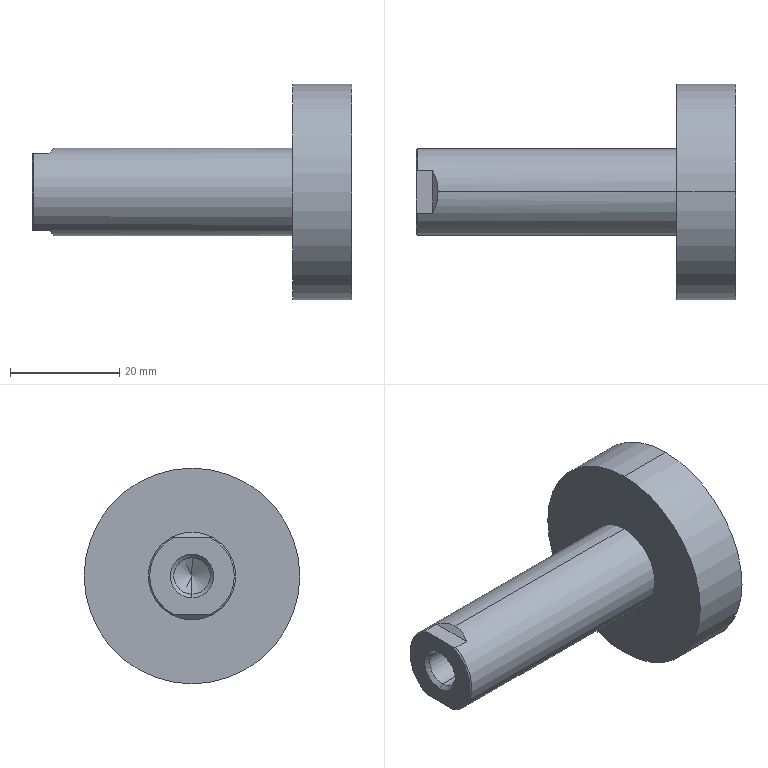Part | SolidWorks | features MBimport 1 | 1 solid | 19 faces | box 58.5 x 39.5 x 39.5 mm | volume 22261 mm3 | plane 7 | cylinder 6 | cone 6 | commonest cylinder face diameters 6.647 x2 16 x2 39.5 x2
STEP:
#1=CARTESIAN_POINT('',(-3.,0.,8.));
#2=VERTEX_POINT('',#1);
#3=CARTESIAN_POINT('',(-4.,3.873,7.));
#4=VERTEX_POINT('',#3);
#5=CARTESIAN_POINT('',(-3.,0.,8.));
#6=CARTESIAN_POINT('',(-3.,1.362,8.));
#7=CARTESIAN_POINT('',(-3.341,2.681,7.659));
#8=CARTESIAN_POINT('',(-4.,3.873,7.));
#9=(BOUNDED_CURVE()B_SPLINE_CURVE(3,(#5,#6,#7,#8),.UNSPECIFIED.,.F.,.F.)B_SPLINE_CURVE_WITH_KNOTS((4,4),(0.,0.5054),.UNSPECIFIED.)CURVE()GEOMETRIC_REPRESENTATION_ITEM()RATIONAL_B_SPLINE_CURVE((1.,0.9788,0.9788,1.))REPRESENTATION_ITEM(''));
#10=EDGE_CURVE('',#2,#4,#9,.T.);
#11=ORIENTED_EDGE('',*,*,#10,.F.);
#12=CARTESIAN_POINT('',(40.7,0.,8.));
#13=VERTEX_POINT('',#12);
#14=CARTESIAN_POINT('',(0.,0.,8.));
#15=DIRECTION('',(1.,0.,0.));
#16=VECTOR('',#15,1000.);
#17=LINE('',#14,#16);
#18=EDGE_CURVE('',#2,#13,#17,.T.);
#19=ORIENTED_EDGE('',*,*,#18,.T.);
#20=CARTESIAN_POINT('',(40.7,0.,-8.));
#21=VERTEX_POINT('',#20);
#22=CARTESIAN_POINT('',(40.7,0.,0.));
#23=DIRECTION('',(1.,0.,0.));
#24=DIRECTION('',(0.,0.,-1.));
#25=AXIS2_PLACEMENT_3D('',#22,#23,#24);
#26=CIRCLE('',#25,8.);
#27=EDGE_CURVE('',#21,#13,#26,.T.);
#28=ORIENTED_EDGE('',*,*,#27,.F.);
#29=CARTESIAN_POINT('',(-3.,0.,-8.));
#30=VERTEX_POINT('',#29);
#31=CARTESIAN_POINT('',(0.,0.,-8.));
#32=DIRECTION('',(1.,0.,0.));
#33=VECTOR('',#32,1000.);
#34=LINE('',#31,#33);
#35=EDGE_CURVE('',#30,#21,#34,.T.);
#36=ORIENTED_EDGE('',*,*,#35,.F.);
#37=CARTESIAN_POINT('',(-4.,3.873,-7.));
#38=VERTEX_POINT('',#37);
#39=CARTESIAN_POINT('',(-4.,3.873,-7.));
#40=CARTESIAN_POINT('',(-3.341,2.681,-7.659));
#41=CARTESIAN_POINT('',(-3.,1.362,-8.));
#42=CARTESIAN_POINT('',(-3.,0.,-8.));
#43=(BOUNDED_CURVE()B_SPLINE_CURVE(3,(#39,#40,#41,#42),.UNSPECIFIED.,.F.,.F.)B_SPLINE_CURVE_WITH_KNOTS((4,4),(5.778,6.283),.UNSPECIFIED.)CURVE()GEOMETRIC_REPRESENTATION_ITEM()RATIONAL_B_SPLINE_CURVE((1.,0.9788,0.9788,1.))REPRESENTATION_ITEM(''));
#44=EDGE_CURVE('',#38,#30,#43,.T.);
#45=ORIENTED_EDGE('',*,*,#44,.F.);
#46=CARTESIAN_POINT('',(-6.75,3.873,-7.));
#47=VERTEX_POINT('',#46);
#48=CARTESIAN_POINT('',(0.,3.873,-7.));
#49=DIRECTION('',(1.,0.,0.));
#50=VECTOR('',#49,1000.);
#51=LINE('',#48,#50);
#52=EDGE_CURVE('',#47,#38,#51,.T.);
#53=ORIENTED_EDGE('',*,*,#52,.F.);
#54=CARTESIAN_POINT('',(-6.75,3.873,7.));
#55=VERTEX_POINT('',#54);
#56=CARTESIAN_POINT('',(-6.75,0.,0.));
#57=DIRECTION('',(1.,0.,0.));
#58=DIRECTION('',(0.,0.,-1.));
#59=AXIS2_PLACEMENT_3D('',#56,#57,#58);
#60=CIRCLE('',#59,8.);
#61=EDGE_CURVE('',#47,#55,#60,.T.);
#62=ORIENTED_EDGE('',*,*,#61,.T.);
#63=CARTESIAN_POINT('',(0.,3.873,7.));
#64=DIRECTION('',(-1.,0.,0.));
#65=VECTOR('',#64,1000.);
#66=LINE('',#63,#65);
#67=EDGE_CURVE('',#4,#55,#66,.T.);
#68=ORIENTED_EDGE('',*,*,#67,.F.);
#69=EDGE_LOOP('',(#11,#19,#28,#36,#45,#53,#62,#68));
#70=FACE_OUTER_BOUND('',#69,.T.);
#71=CARTESIAN_POINT('',(0.,0.,0.));
#72=DIRECTION('',(1.,0.,0.));
#73=DIRECTION('',(0.,0.,-1.));
#74=AXIS2_PLACEMENT_3D('',#71,#72,#73);
#75=CYLINDRICAL_SURFACE('',#74,8.);
#76=ADVANCED_FACE('',(#70),#75,.T.);
#77=CARTESIAN_POINT('',(40.7,0.,-19.75));
#78=VERTEX_POINT('',#77);
#79=CARTESIAN_POINT('',(40.7,0.,19.75));
#80=VERTEX_POINT('',#79);
#81=CARTESIAN_POINT('',(40.7,0.,0.));
#82=DIRECTION('',(1.,0.,0.));
#83=DIRECTION('',(0.,0.,-1.));
#84=AXIS2_PLACEMENT_3D('',#81,#82,#83);
#85=CIRCLE('',#84,19.75);
#86=EDGE_CURVE('',#78,#80,#85,.T.);
#87=ORIENTED_EDGE('',*,*,#86,.T.);
#88=CARTESIAN_POINT('',(51.5,0.,19.75));
#89=VERTEX_POINT('',#88);
#90=CARTESIAN_POINT('',(51.5,0.,19.75));
#91=DIRECTION('',(1.,0.,0.));
#92=VECTOR('',#91,1000.);
#93=LINE('',#90,#92);
#94=EDGE_CURVE('',#80,#89,#93,.T.);
#95=ORIENTED_EDGE('',*,*,#94,.T.);
#96=CARTESIAN_POINT('',(51.5,0.,-19.75));
#97=VERTEX_POINT('',#96);
#98=CARTESIAN_POINT('',(51.5,0.,0.));
#99=DIRECTION('',(1.,0.,0.));
#100=DIRECTION('',(0.,0.,-1.));
#101=AXIS2_PLACEMENT_3D('',#98,#99,#100);
#102=CIRCLE('',#101,19.75);
#103=EDGE_CURVE('',#97,#89,#102,.T.);
#104=ORIENTED_EDGE('',*,*,#103,.F.);
#105=CARTESIAN_POINT('',(51.5,0.,-19.75));
#106=DIRECTION('',(1.,0.,0.));
#107=VECTOR('',#106,1000.);
#108=LINE('',#105,#107);
#109=EDGE_CURVE('',#78,#97,#108,.T.);
#110=ORIENTED_EDGE('',*,*,#109,.F.);
#111=EDGE_LOOP('',(#87,#95,#104,#110));
#112=FACE_OUTER_BOUND('',#111,.T.);
#113=CARTESIAN_POINT('',(51.5,0.,0.));
#114=DIRECTION('',(1.,0.,0.));
#115=DIRECTION('',(0.,0.,-1.));
#116=AXIS2_PLACEMENT_3D('',#113,#114,#115);
#117=CYLINDRICAL_SURFACE('',#116,19.75);
#118=ADVANCED_FACE('',(#112),#117,.T.);
#119=CARTESIAN_POINT('',(-6.324,0.,3.324));
#120=VERTEX_POINT('',#119);
#121=CARTESIAN_POINT('',(-6.324,0.,-3.324));
#122=VERTEX_POINT('',#121);
#123=CARTESIAN_POINT('',(-6.324,0.,0.));
#124=DIRECTION('',(1.,0.,0.));
#125=DIRECTION('',(0.,0.,-1.));
#126=AXIS2_PLACEMENT_3D('',#123,#124,#125);
#127=CIRCLE('',#126,3.324);
#128=EDGE_CURVE('',#120,#122,#127,.T.);
#129=ORIENTED_EDGE('',*,*,#128,.T.);
#130=CARTESIAN_POINT('',(-7.,0.,-4.));
#131=VERTEX_POINT('',#130);
#132=CARTESIAN_POINT('',(-7.,0.,-4.));
#133=DIRECTION('',(-0.7071,0.,-0.7071));
#134=VECTOR('',#133,1000.);
#135=LINE('',#132,#134);
#136=EDGE_CURVE('',#122,#131,#135,.T.);
#137=ORIENTED_EDGE('',*,*,#136,.T.);
#138=CARTESIAN_POINT('',(-7.,0.,4.));
#139=VERTEX_POINT('',#138);
#140=CARTESIAN_POINT('',(-7.,0.,0.));
#141=DIRECTION('',(1.,0.,0.));
#142=DIRECTION('',(0.,0.,-1.));
#143=AXIS2_PLACEMENT_3D('',#140,#141,#142);
#144=CIRCLE('',#143,4.);
#145=EDGE_CURVE('',#139,#131,#144,.T.);
#146=ORIENTED_EDGE('',*,*,#145,.F.);
#147=CARTESIAN_POINT('',(-7.,0.,4.));
#148=DIRECTION('',(-0.7071,0.,0.7071));
#149=VECTOR('',#148,1000.);
#150=LINE('',#147,#149);
#151=EDGE_CURVE('',#120,#139,#150,.T.);
#152=ORIENTED_EDGE('',*,*,#151,.F.);
#153=EDGE_LOOP('',(#129,#137,#146,#152));
#154=FACE_OUTER_BOUND('',#153,.T.);
#155=CARTESIAN_POINT('',(-7.,0.,0.));
#156=DIRECTION('',(-1.,0.,0.));
#157=DIRECTION('',(0.,0.,1.));
#158=AXIS2_PLACEMENT_3D('',#155,#156,#157);
#159=CONICAL_SURFACE('',#158,4.,0.7854);
#160=ADVANCED_FACE('',(#154),#159,.F.);
#161=ORIENTED_EDGE('',*,*,#128,.F.);
#162=CARTESIAN_POINT('',(7.4,0.,3.324));
#163=VERTEX_POINT('',#162);
#164=CARTESIAN_POINT('',(9.319,0.,3.324));
#165=DIRECTION('',(1.,0.,0.));
#166=VECTOR('',#165,1000.);
#167=LINE('',#164,#166);
#168=EDGE_CURVE('',#120,#163,#167,.T.);
#169=ORIENTED_EDGE('',*,*,#168,.T.);
#170=CARTESIAN_POINT('',(7.4,0.,-3.324));
#171=VERTEX_POINT('',#170);
#172=CARTESIAN_POINT('',(7.4,0.,0.));
#173=DIRECTION('',(1.,0.,0.));
#174=DIRECTION('',(0.,0.,-1.));
#175=AXIS2_PLACEMENT_3D('',#172,#173,#174);
#176=CIRCLE('',#175,3.324);
#177=EDGE_CURVE('',#163,#171,#176,.T.);
#178=ORIENTED_EDGE('',*,*,#177,.T.);
#179=CARTESIAN_POINT('',(9.319,0.,-3.324));
#180=DIRECTION('',(1.,0.,0.));
#181=VECTOR('',#180,1000.);
#182=LINE('',#179,#181);
#183=EDGE_CURVE('',#122,#171,#182,.T.);
#184=ORIENTED_EDGE('',*,*,#183,.F.);
#185=EDGE_LOOP('',(#161,#169,#178,#184));
#186=FACE_OUTER_BOUND('',#185,.T.);
#187=CARTESIAN_POINT('',(9.319,0.,0.));
#188=DIRECTION('',(1.,0.,0.));
#189=DIRECTION('',(0.,0.,-1.));
#190=AXIS2_PLACEMENT_3D('',#187,#188,#189);
#191=CYLINDRICAL_SURFACE('',#190,3.324);
#192=ADVANCED_FACE('',(#186),#191,.F.);
#193=CARTESIAN_POINT('',(9.319,0.,0.));
#194=VERTEX_POINT('',#193);
#195=CARTESIAN_POINT('',(7.4,0.,3.324));
#196=DIRECTION('',(-0.5,0.,0.866));
#197=VECTOR('',#196,1000.);
#198=LINE('',#195,#197);
#199=EDGE_CURVE('',#194,#163,#198,.T.);
#200=ORIENTED_EDGE('',*,*,#199,.F.);
#201=CARTESIAN_POINT('',(7.4,0.,-3.324));
#202=DIRECTION('',(-0.5,0.,-0.866));
#203=VECTOR('',#202,1000.);
#204=LINE('',#201,#203);
#205=EDGE_CURVE('',#194,#171,#204,.T.);
#206=ORIENTED_EDGE('',*,*,#205,.T.);
#207=ORIENTED_EDGE('',*,*,#177,.F.);
#208=EDGE_LOOP('',(#200,#206,#207));
#209=FACE_OUTER_BOUND('',#208,.T.);
#210=CARTESIAN_POINT('',(7.4,0.,0.));
#211=DIRECTION('',(-1.,0.,0.));
#212=DIRECTION('',(0.,0.,1.));
#213=AXIS2_PLACEMENT_3D('',#210,#211,#212);
#214=CONICAL_SURFACE('',#213,3.324,1.047);
#215=ADVANCED_FACE('',(#209),#214,.F.);
#216=ORIENTED_EDGE('',*,*,#205,.F.);
#217=ORIENTED_EDGE('',*,*,#199,.T.);
#218=CARTESIAN_POINT('',(7.4,0.,0.));
#219=DIRECTION('',(1.,0.,0.));
#220=DIRECTION('',(0.,0.,-1.));
#221=AXIS2_PLACEMENT_3D('',#218,#219,#220);
#222=CIRCLE('',#221,3.324);
#223=EDGE_CURVE('',#171,#163,#222,.T.);
#224=ORIENTED_EDGE('',*,*,#223,.F.);
#225=EDGE_LOOP('',(#216,#217,#224));
#226=FACE_OUTER_BOUND('',#225,.T.);
#227=CARTESIAN_POINT('',(7.4,0.,0.));
#228=DIRECTION('',(-1.,0.,0.));
#229=DIRECTION('',(0.,0.,1.));
#230=AXIS2_PLACEMENT_3D('',#227,#228,#229);
#231=CONICAL_SURFACE('',#230,3.324,1.047);
#232=ADVANCED_FACE('',(#226),#231,.F.);
#233=ORIENTED_EDGE('',*,*,#168,.F.);
#234=CARTESIAN_POINT('',(-6.324,0.,0.));
#235=DIRECTION('',(1.,0.,0.));
#236=DIRECTION('',(0.,0.,-1.));
#237=AXIS2_PLACEMENT_3D('',#234,#235,#236);
#238=CIRCLE('',#237,3.324);
#239=EDGE_CURVE('',#122,#120,#238,.T.);
#240=ORIENTED_EDGE('',*,*,#239,.F.);
#241=ORIENTED_EDGE('',*,*,#183,.T.);
#242=ORIENTED_EDGE('',*,*,#223,.T.);
#243=EDGE_LOOP('',(#233,#240,#241,#242));
#244=FACE_OUTER_BOUND('',#243,.T.);
#245=CARTESIAN_POINT('',(9.319,0.,0.));
#246=DIRECTION('',(1.,0.,0.));
#247=DIRECTION('',(0.,0.,-1.));
#248=AXIS2_PLACEMENT_3D('',#245,#246,#247);
#249=CYLINDRICAL_SURFACE('',#248,3.324);
#250=ADVANCED_FACE('',(#244),#249,.F.);
#251=ORIENTED_EDGE('',*,*,#136,.F.);
#252=ORIENTED_EDGE('',*,*,#239,.T.);
#253=ORIENTED_EDGE('',*,*,#151,.T.);
#254=CARTESIAN_POINT('',(-7.,0.,0.));
#255=DIRECTION('',(1.,0.,0.));
#256=DIRECTION('',(0.,0.,-1.));
#257=AXIS2_PLACEMENT_3D('',#254,#255,#256);
#258=CIRCLE('',#257,4.);
#259=EDGE_CURVE('',#131,#139,#258,.T.);
#260=ORIENTED_EDGE('',*,*,#259,.F.);
#261=EDGE_LOOP('',(#251,#252,#253,#260));
#262=FACE_OUTER_BOUND('',#261,.T.);
#263=CARTESIAN_POINT('',(-7.,0.,0.));
#264=DIRECTION('',(-1.,0.,0.));
#265=DIRECTION('',(0.,0.,1.));
#266=AXIS2_PLACEMENT_3D('',#263,#264,#265);
#267=CONICAL_SURFACE('',#266,4.,0.7854);
#268=ADVANCED_FACE('',(#262),#267,.F.);
#269=CARTESIAN_POINT('',(-7.,-3.326,7.));
#270=VERTEX_POINT('',#269);
#271=CARTESIAN_POINT('',(-6.75,-3.873,7.));
#272=VERTEX_POINT('',#271);
#273=CARTESIAN_POINT('',(-7.,-3.326,7.));
#274=CARTESIAN_POINT('',(-6.921,-3.51,7.));
#275=CARTESIAN_POINT('',(-6.837,-3.692,7.));
#276=CARTESIAN_POINT('',(-6.75,-3.873,7.));
#277=B_SPLINE_CURVE_WITH_KNOTS('',3,(#273,#274,#275,#276),.UNSPECIFIED.,.F.,.F.,(4,4),(0.007395,0.007986),.UNSPECIFIED.);
#278=EDGE_CURVE('',#270,#272,#277,.T.);
#279=ORIENTED_EDGE('',*,*,#278,.T.);
#280=CARTESIAN_POINT('',(-4.,-3.873,7.));
#281=VERTEX_POINT('',#280);
#282=CARTESIAN_POINT('',(0.,-3.873,7.));
#283=DIRECTION('',(1.,0.,0.));
#284=VECTOR('',#283,1000.);
#285=LINE('',#282,#284);
#286=EDGE_CURVE('',#272,#281,#285,.T.);
#287=ORIENTED_EDGE('',*,*,#286,.T.);
#288=CARTESIAN_POINT('',(-4.,14.,7.));
#289=DIRECTION('',(0.,-1.,0.));
#290=VECTOR('',#289,1000.);
#291=LINE('',#288,#290);
#292=EDGE_CURVE('',#4,#281,#291,.T.);
#293=ORIENTED_EDGE('',*,*,#292,.F.);
#294=ORIENTED_EDGE('',*,*,#67,.T.);
#295=CARTESIAN_POINT('',(-7.,3.326,7.));
#296=VERTEX_POINT('',#295);
#297=CARTESIAN_POINT('',(-6.75,3.873,7.));
#298=CARTESIAN_POINT('',(-6.838,3.692,7.));
#299=CARTESIAN_POINT('',(-6.921,3.51,7.));
#300=CARTESIAN_POINT('',(-7.,3.326,7.));
#301=B_SPLINE_CURVE_WITH_KNOTS('',3,(#297,#298,#299,#300),.UNSPECIFIED.,.F.,.F.,(4,4),(0.000001583,0.0005965),.UNSPECIFIED.);
#302=EDGE_CURVE('',#55,#296,#301,.T.);
#303=ORIENTED_EDGE('',*,*,#302,.T.);
#304=CARTESIAN_POINT('',(-7.,14.,7.));
#305=DIRECTION('',(0.,-1.,0.));
#306=VECTOR('',#305,1000.);
#307=LINE('',#304,#306);
#308=EDGE_CURVE('',#296,#270,#307,.T.);
#309=ORIENTED_EDGE('',*,*,#308,.T.);
#310=EDGE_LOOP('',(#279,#287,#293,#294,#303,#309));
#311=FACE_OUTER_BOUND('',#310,.T.);
#312=CARTESIAN_POINT('',(-4.,14.,7.));
#313=DIRECTION('',(0.,0.,1.));
#314=DIRECTION('',(1.,0.,0.));
#315=AXIS2_PLACEMENT_3D('',#312,#313,#314);
#316=PLANE('',#315);
#317=ADVANCED_FACE('',(#311),#316,.T.);
#318=CARTESIAN_POINT('',(-4.,-3.873,7.));
#319=CARTESIAN_POINT('',(-3.341,-2.681,7.659));
#320=CARTESIAN_POINT('',(-3.,-1.362,8.));
#321=CARTESIAN_POINT('',(-3.,0.,8.));
#322=(BOUNDED_CURVE()B_SPLINE_CURVE(3,(#318,#319,#320,#321),.UNSPECIFIED.,.F.,.F.)B_SPLINE_CURVE_WITH_KNOTS((4,4),(5.778,6.283),.UNSPECIFIED.)CURVE()GEOMETRIC_REPRESENTATION_ITEM()RATIONAL_B_SPLINE_CURVE((1.,0.9788,0.9788,1.))REPRESENTATION_ITEM(''));
#323=EDGE_CURVE('',#281,#2,#322,.T.);
#324=ORIENTED_EDGE('',*,*,#323,.T.);
#325=ORIENTED_EDGE('',*,*,#10,.T.);
#326=ORIENTED_EDGE('',*,*,#292,.T.);
#327=EDGE_LOOP('',(#324,#325,#326));
#328=FACE_OUTER_BOUND('',#327,.T.);
#329=CARTESIAN_POINT('',(1.,14.,12.));
#330=DIRECTION('',(-0.7071,0.,0.7071));
#331=DIRECTION('',(0.,1.,0.));
#332=AXIS2_PLACEMENT_3D('',#329,#330,#331);
#333=PLANE('',#332);
#334=ADVANCED_FACE('',(#328),#333,.T.);
#335=CARTESIAN_POINT('',(-7.,3.326,-7.));
#336=VERTEX_POINT('',#335);
#337=CARTESIAN_POINT('',(-7.,3.326,-7.));
#338=CARTESIAN_POINT('',(-6.921,3.51,-7.));
#339=CARTESIAN_POINT('',(-6.837,3.692,-7.));
#340=CARTESIAN_POINT('',(-6.75,3.873,-7.));
#341=B_SPLINE_CURVE_WITH_KNOTS('',3,(#337,#338,#339,#340),.UNSPECIFIED.,.F.,.F.,(4,4),(0.007395,0.007986),.UNSPECIFIED.);
#342=EDGE_CURVE('',#336,#47,#341,.T.);
#343=ORIENTED_EDGE('',*,*,#342,.T.);
#344=ORIENTED_EDGE('',*,*,#52,.T.);
#345=CARTESIAN_POINT('',(-4.,-3.873,-7.));
#346=VERTEX_POINT('',#345);
#347=CARTESIAN_POINT('',(-4.,14.,-7.));
#348=DIRECTION('',(0.,-1.,0.));
#349=VECTOR('',#348,1000.);
#350=LINE('',#347,#349);
#351=EDGE_CURVE('',#38,#346,#350,.T.);
#352=ORIENTED_EDGE('',*,*,#351,.T.);
#353=CARTESIAN_POINT('',(-6.75,-3.873,-7.));
#354=VERTEX_POINT('',#353);
#355=CARTESIAN_POINT('',(0.,-3.873,-7.));
#356=DIRECTION('',(-1.,0.,0.));
#357=VECTOR('',#356,1000.);
#358=LINE('',#355,#357);
#359=EDGE_CURVE('',#346,#354,#358,.T.);
#360=ORIENTED_EDGE('',*,*,#359,.T.);
#361=CARTESIAN_POINT('',(-7.,-3.326,-7.));
#362=VERTEX_POINT('',#361);
#363=CARTESIAN_POINT('',(-6.75,-3.873,-7.));
#364=CARTESIAN_POINT('',(-6.838,-3.692,-7.));
#365=CARTESIAN_POINT('',(-6.921,-3.51,-7.));
#366=CARTESIAN_POINT('',(-7.,-3.326,-7.));
#367=B_SPLINE_CURVE_WITH_KNOTS('',3,(#363,#364,#365,#366),.UNSPECIFIED.,.F.,.F.,(4,4),(0.000001583,0.0005965),.UNSPECIFIED.);
#368=EDGE_CURVE('',#354,#362,#367,.T.);
#369=ORIENTED_EDGE('',*,*,#368,.T.);
#370=CARTESIAN_POINT('',(-7.,14.,-7.));
#371=DIRECTION('',(0.,-1.,0.));
#372=VECTOR('',#371,1000.);
#373=LINE('',#370,#372);
#374=EDGE_CURVE('',#336,#362,#373,.T.);
#375=ORIENTED_EDGE('',*,*,#374,.F.);
#376=EDGE_LOOP('',(#343,#344,#352,#360,#369,#375));
#377=FACE_OUTER_BOUND('',#376,.T.);
#378=CARTESIAN_POINT('',(-7.,14.,-7.));
#379=DIRECTION('',(0.,0.,-1.));
#380=DIRECTION('',(0.,-1.,0.));
#381=AXIS2_PLACEMENT_3D('',#378,#379,#380);
#382=PLANE('',#381);
#383=ADVANCED_FACE('',(#377),#382,.T.);
#384=ORIENTED_EDGE('',*,*,#44,.T.);
#385=CARTESIAN_POINT('',(-3.,0.,-8.));
#386=CARTESIAN_POINT('',(-3.,-1.362,-8.));
#387=CARTESIAN_POINT('',(-3.341,-2.681,-7.659));
#388=CARTESIAN_POINT('',(-4.,-3.873,-7.));
#389=(BOUNDED_CURVE()B_SPLINE_CURVE(3,(#385,#386,#387,#388),.UNSPECIFIED.,.F.,.F.)B_SPLINE_CURVE_WITH_KNOTS((4,4),(0.,0.5054),.UNSPECIFIED.)CURVE()GEOMETRIC_REPRESENTATION_ITEM()RATIONAL_B_SPLINE_CURVE((1.,0.9788,0.9788,1.))REPRESENTATION_ITEM(''));
#390=EDGE_CURVE('',#30,#346,#389,.T.);
#391=ORIENTED_EDGE('',*,*,#390,.T.);
#392=ORIENTED_EDGE('',*,*,#351,.F.);
#393=EDGE_LOOP('',(#384,#391,#392));
#394=FACE_OUTER_BOUND('',#393,.T.);
#395=CARTESIAN_POINT('',(-4.,14.,-7.));
#396=DIRECTION('',(-0.7071,0.,-0.7071));
#397=DIRECTION('',(-0.7071,0.,0.7071));
#398=AXIS2_PLACEMENT_3D('',#395,#396,#397);
#399=PLANE('',#398);
#400=ADVANCED_FACE('',(#394),#399,.T.);
#401=ORIENTED_EDGE('',*,*,#103,.T.);
#402=CARTESIAN_POINT('',(51.5,0.,0.));
#403=DIRECTION('',(1.,0.,0.));
#404=DIRECTION('',(0.,0.,-1.));
#405=AXIS2_PLACEMENT_3D('',#402,#403,#404);
#406=CIRCLE('',#405,19.75);
#407=EDGE_CURVE('',#89,#97,#406,.T.);
#408=ORIENTED_EDGE('',*,*,#407,.T.);
#409=EDGE_LOOP('',(#401,#408));
#410=FACE_OUTER_BOUND('',#409,.T.);
#411=CARTESIAN_POINT('',(51.5,19.75,0.));
#412=DIRECTION('',(-1.,0.,0.));
#413=DIRECTION('',(0.,0.,1.));
#414=AXIS2_PLACEMENT_3D('',#411,#412,#413);
#415=PLANE('',#414);
#416=ADVANCED_FACE('',(#410),#415,.F.);
#417=ORIENTED_EDGE('',*,*,#94,.F.);
#418=CARTESIAN_POINT('',(40.7,0.,0.));
#419=DIRECTION('',(1.,0.,0.));
#420=DIRECTION('',(0.,0.,-1.));
#421=AXIS2_PLACEMENT_3D('',#418,#419,#420);
#422=CIRCLE('',#421,19.75);
#423=EDGE_CURVE('',#80,#78,#422,.T.);
#424=ORIENTED_EDGE('',*,*,#423,.T.);
#425=ORIENTED_EDGE('',*,*,#109,.T.);
#426=ORIENTED_EDGE('',*,*,#407,.F.);
#427=EDGE_LOOP('',(#417,#424,#425,#426));
#428=FACE_OUTER_BOUND('',#427,.T.);
#429=CARTESIAN_POINT('',(51.5,0.,0.));
#430=DIRECTION('',(1.,0.,0.));
#431=DIRECTION('',(0.,0.,-1.));
#432=AXIS2_PLACEMENT_3D('',#429,#430,#431);
#433=CYLINDRICAL_SURFACE('',#432,19.75);
#434=ADVANCED_FACE('',(#428),#433,.T.);
#435=ORIENTED_EDGE('',*,*,#27,.T.);
#436=CARTESIAN_POINT('',(40.7,0.,0.));
#437=DIRECTION('',(1.,0.,0.));
#438=DIRECTION('',(0.,0.,-1.));
#439=AXIS2_PLACEMENT_3D('',#436,#437,#438);
#440=CIRCLE('',#439,8.);
#441=EDGE_CURVE('',#13,#21,#440,.T.);
#442=ORIENTED_EDGE('',*,*,#441,.T.);
#443=EDGE_LOOP('',(#435,#442));
#444=FACE_BOUND('',#443,.T.);
#445=ORIENTED_EDGE('',*,*,#86,.F.);
#446=ORIENTED_EDGE('',*,*,#423,.F.);
#447=EDGE_LOOP('',(#445,#446));
#448=FACE_OUTER_BOUND('',#447,.T.);
#449=CARTESIAN_POINT('',(40.7,8.,0.));
#450=DIRECTION('',(1.,0.,0.));
#451=DIRECTION('',(0.,1.,0.));
#452=AXIS2_PLACEMENT_3D('',#449,#450,#451);
#453=PLANE('',#452);
#454=ADVANCED_FACE('',(#444,#448),#453,.F.);
#455=ORIENTED_EDGE('',*,*,#18,.F.);
#456=ORIENTED_EDGE('',*,*,#323,.F.);
#457=ORIENTED_EDGE('',*,*,#286,.F.);
#458=CARTESIAN_POINT('',(-6.75,0.,0.));
#459=DIRECTION('',(1.,0.,0.));
#460=DIRECTION('',(0.,0.,-1.));
#461=AXIS2_PLACEMENT_3D('',#458,#459,#460);
#462=CIRCLE('',#461,8.);
#463=EDGE_CURVE('',#272,#354,#462,.T.);
#464=ORIENTED_EDGE('',*,*,#463,.T.);
#465=ORIENTED_EDGE('',*,*,#359,.F.);
#466=ORIENTED_EDGE('',*,*,#390,.F.);
#467=ORIENTED_EDGE('',*,*,#35,.T.);
#468=ORIENTED_EDGE('',*,*,#441,.F.);
#469=EDGE_LOOP('',(#455,#456,#457,#464,#465,#466,#467,#468));
#470=FACE_OUTER_BOUND('',#469,.T.);
#471=CARTESIAN_POINT('',(0.,0.,0.));
#472=DIRECTION('',(1.,0.,0.));
#473=DIRECTION('',(0.,0.,-1.));
#474=AXIS2_PLACEMENT_3D('',#471,#472,#473);
#475=CYLINDRICAL_SURFACE('',#474,8.);
#476=ADVANCED_FACE('',(#470),#475,.T.);
#477=ORIENTED_EDGE('',*,*,#342,.F.);
#478=CARTESIAN_POINT('',(-7.,0.,0.));
#479=DIRECTION('',(1.,0.,0.));
#480=DIRECTION('',(0.,0.,-1.));
#481=AXIS2_PLACEMENT_3D('',#478,#479,#480);
#482=CIRCLE('',#481,7.75);
#483=EDGE_CURVE('',#336,#296,#482,.T.);
#484=ORIENTED_EDGE('',*,*,#483,.T.);
#485=ORIENTED_EDGE('',*,*,#302,.F.);
#486=ORIENTED_EDGE('',*,*,#61,.F.);
#487=EDGE_LOOP('',(#477,#484,#485,#486));
#488=FACE_OUTER_BOUND('',#487,.T.);
#489=CARTESIAN_POINT('',(-7.,0.,0.));
#490=DIRECTION('',(1.,0.,0.));
#491=DIRECTION('',(0.,0.,-1.));
#492=AXIS2_PLACEMENT_3D('',#489,#490,#491);
#493=CONICAL_SURFACE('',#492,7.75,0.7854);
#494=ADVANCED_FACE('',(#488),#493,.T.);
#495=ORIENTED_EDGE('',*,*,#278,.F.);
#496=CARTESIAN_POINT('',(-7.,0.,0.));
#497=DIRECTION('',(1.,0.,0.));
#498=DIRECTION('',(0.,0.,-1.));
#499=AXIS2_PLACEMENT_3D('',#496,#497,#498);
#500=CIRCLE('',#499,7.75);
#501=EDGE_CURVE('',#270,#362,#500,.T.);
#502=ORIENTED_EDGE('',*,*,#501,.T.);
#503=ORIENTED_EDGE('',*,*,#368,.F.);
#504=ORIENTED_EDGE('',*,*,#463,.F.);
#505=EDGE_LOOP('',(#495,#502,#503,#504));
#506=FACE_OUTER_BOUND('',#505,.T.);
#507=CARTESIAN_POINT('',(-7.,0.,0.));
#508=DIRECTION('',(1.,0.,0.));
#509=DIRECTION('',(0.,0.,-1.));
#510=AXIS2_PLACEMENT_3D('',#507,#508,#509);
#511=CONICAL_SURFACE('',#510,7.75,0.7854);
#512=ADVANCED_FACE('',(#506),#511,.T.);
#513=ORIENTED_EDGE('',*,*,#145,.T.);
#514=ORIENTED_EDGE('',*,*,#259,.T.);
#515=EDGE_LOOP('',(#513,#514));
#516=FACE_BOUND('',#515,.T.);
#517=ORIENTED_EDGE('',*,*,#483,.F.);
#518=ORIENTED_EDGE('',*,*,#374,.T.);
#519=ORIENTED_EDGE('',*,*,#501,.F.);
#520=ORIENTED_EDGE('',*,*,#308,.F.);
#521=EDGE_LOOP('',(#517,#518,#519,#520));
#522=FACE_OUTER_BOUND('',#521,.T.);
#523=CARTESIAN_POINT('',(-7.,0.,0.));
#524=DIRECTION('',(1.,0.,0.));
#525=DIRECTION('',(0.,1.,0.));
#526=AXIS2_PLACEMENT_3D('',#523,#524,#525);
#527=PLANE('',#526);
#528=ADVANCED_FACE('',(#516,#522),#527,.F.);
#529=CLOSED_SHELL('',(#76,#118,#160,#192,#215,#232,#250,#268,#317,#334,#383,#400,#416,#434,#454,#476,#494,#512,#528));
#530=MANIFOLD_SOLID_BREP('',#529);
#531=CARTESIAN_POINT('',(0.,0.,0.));
#532=DIRECTION('',(0.,0.,1.));
#533=DIRECTION('',(1.,0.,0.));
#534=AXIS2_PLACEMENT_3D('',#531,#532,#533);
#535=(LENGTH_UNIT()NAMED_UNIT(*)SI_UNIT(.MILLI.,.METRE.));
#536=UNCERTAINTY_MEASURE_WITH_UNIT(LENGTH_MEASURE(0.00001),#535,'','');
#537=(NAMED_UNIT(*)PLANE_ANGLE_UNIT()SI_UNIT($,.RADIAN.));
#538=(NAMED_UNIT(*)SI_UNIT($,.STERADIAN.)SOLID_ANGLE_UNIT());
#539=(GEOMETRIC_REPRESENTATION_CONTEXT(3)GLOBAL_UNCERTAINTY_ASSIGNED_CONTEXT((#536))GLOBAL_UNIT_ASSIGNED_CONTEXT((#535,#537,#538))REPRESENTATION_CONTEXT('',''));
#540=ADVANCED_BREP_SHAPE_REPRESENTATION('',(#530,#534),#539);